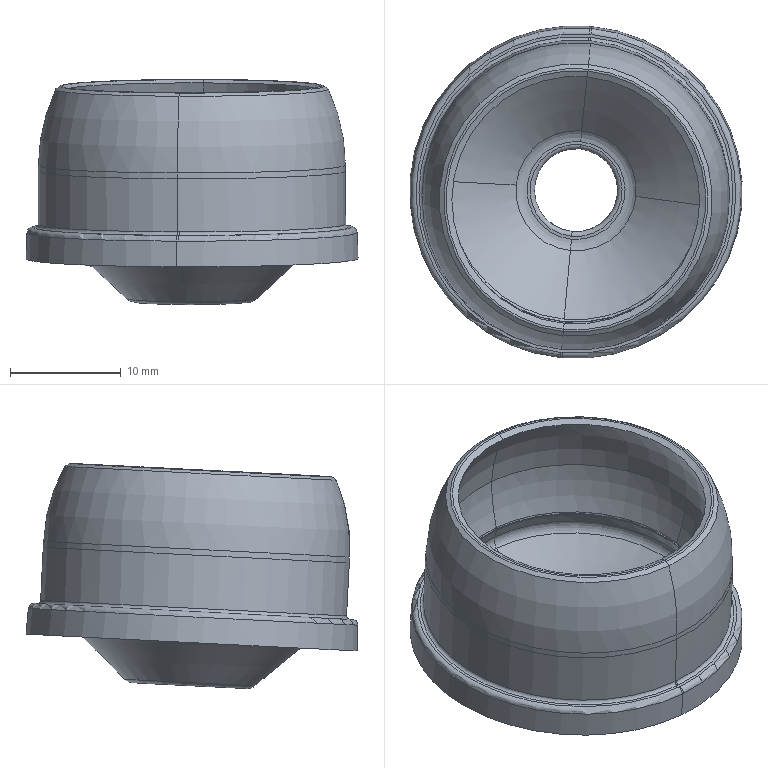Part | SolidWorks | features BaseBody 1 | 1 solid | 64 faces | box 29.983 x 29.981 x 20.298 mm | volume 2883 mm3 | torus 44 | cone 12 | plane 4 | cylinder 4 | commonest cylinder face diameters 7.5 x2 27.7 x2